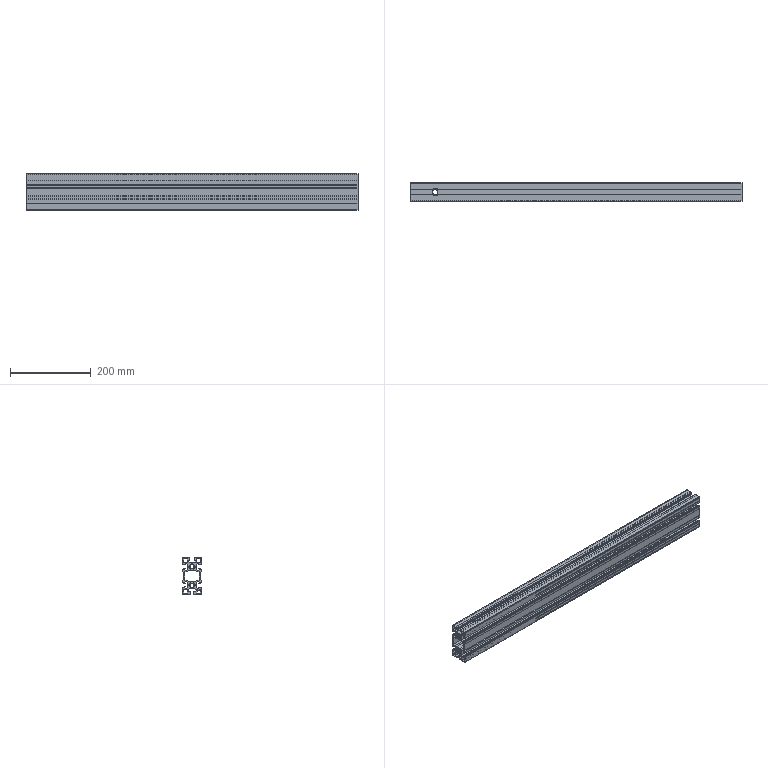Part | STEP file | 1 solid | 401 faces | box 820 x 45 x 90 mm | volume 1189309 mm3 | plane 344 | cylinder 57 | commonest cylinder face diameters 10 x36 13 x14 2 x4 19 x3